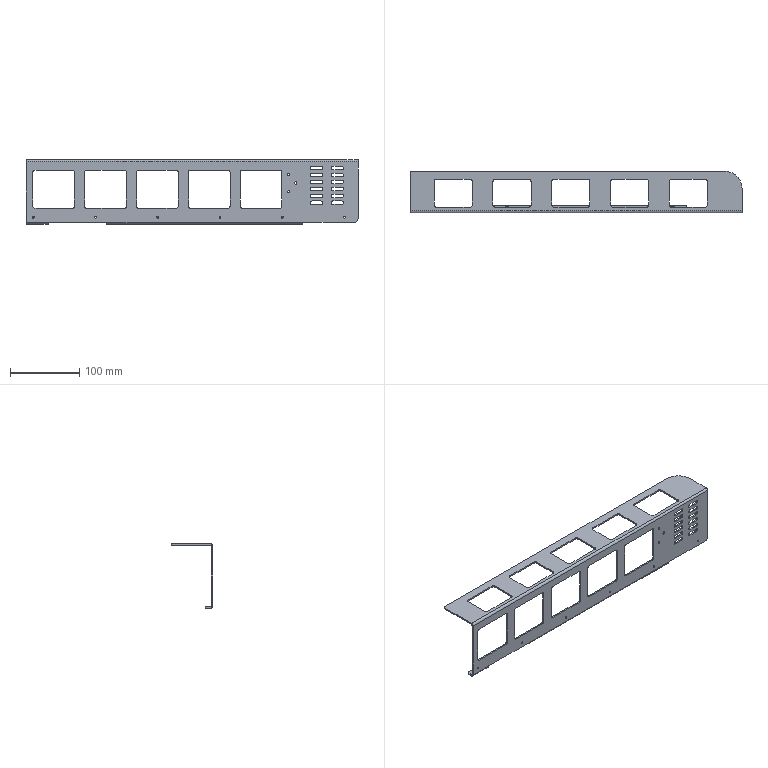Part | NX | features BREP 1 | 1 solid | 197 faces | box 480 x 60 x 93 mm | volume 90767 mm3 | cylinder 101 | plane 96 | commonest cylinder face diameters 6 x43 5 x32 2.5 x12 3.3 x6 2 x3 4 x3